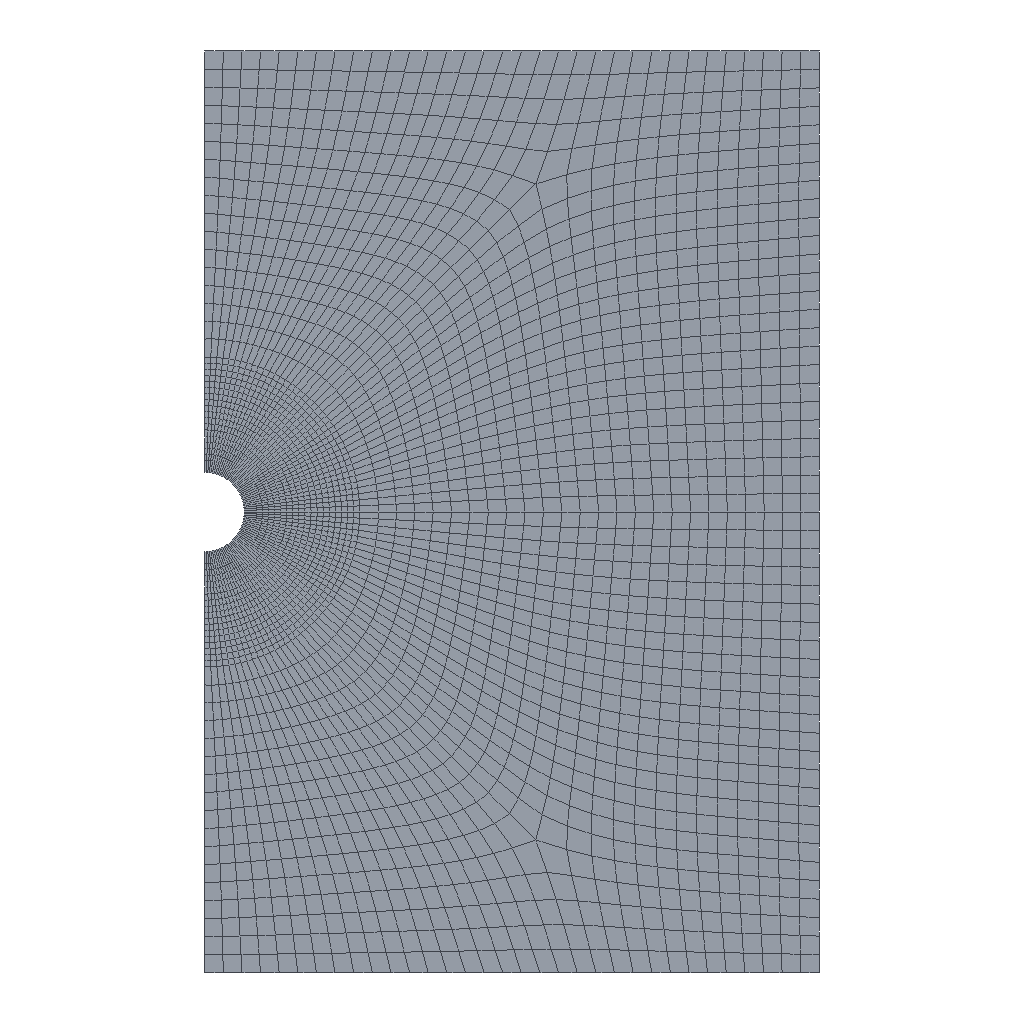Simulation study | abaqus
Set-up summary:
category,name,step,type,value,unit,region
solver,abaqus
solver,version,,,Abaqus/Standard 2020
units,not stated in the deck,,not stated
analysis,deck,,geostatic,geostatic
load_step,geo,geo,geostatic
load_step,Step-1,Step-1,soils
load_step,requested,,,2
mesh,nodes,,,3503
mesh,elements,,,3349
element_type,CPE4P,,plane,3330
element_type,COH2D4P,,cohesive,19
load,load commands in deck,,count,4
bc,support commands in deck,,count,4
material,COH,,in results
material,COH-0,,in results
material,ROCK,,in results
check,setup vs results,,match,"per instance, exact: element labels, types and connectivity; labels of the nodes the elements use; coordinates of those nodes at SINGLE_PRECISION in 1 of 1 instance(s)"
Abaqus input file, long lists of numbers shortened:
*Heading
** Job name: Job-2 Model name: Model-1-Copy-Copy
** Generated by: Abaqus/CAE 2020
*Preprint, echo=NO, model=NO, history=NO, contact=NO
**
** PARTS
**
*Part, name=work
*Node
      1,   25.206,           0.
      2,   6.441,           0.
** (3501 more lines like these left out)
*Element, type=CPE4P
  1,    1, 3466,  390,  125
  2, 3466, 3467,  391,  390
** (3328 more lines like these left out)
*Element, type=COH2D4P
3331,    1,   12, 3466,    1,    1, 3485
3332,   12,   13, 3467, 3466, 3485, 3486
** (17 more lines like these left out)
*Nset, nset=Set-111
    1,    2,    3,    4,    5,    6,   12,   13,   14,   15,   16,   17,   18,   19,   20,   21
   22,   23,   24,   25,   26,   27,   28,   29,   30,   31,   32,   33,   34,   35,   36,   37
** (101 more lines like these left out)
*Elset, elset=Set-111, generate
    1,  1520,     1
*Nset, nset=Set-120, generate
    1,  3484,     1
*Elset, elset=Set-120, generate
    1,  3330,     1
*Nset, nset=CohesiveSeam-2-TopNodes
    1, 3466, 3467, 3468, 3469, 3470, 3471, 3472, 3473, 3474, 3475, 3476, 3477, 3478, 3479, 3480
 3481, 3482, 3483, 3484
*Nset, nset=CohesiveSeam-2-BottomNodes
  1,  2, 12, 13, 14, 15, 16, 17, 18, 19, 20, 21, 22, 23, 24, 25
 26, 27, 28, 29
*Nset, nset=CohesiveSeam-2-MidNodes
    1, 3485, 3486, 3487, 3488, 3489, 3490, 3491, 3492, 3493, 3494, 3495, 3496, 3497, 3498, 3499
 3500, 3501, 3502, 3503
*Elset, elset=ele-3336-plug
 3336,
*Nset, nset=node-weiyi-0
   17, 3471, 3490
*Elset, elset=coh-shengyu
 3331, 3332, 3333, 3334, 3335, 3337, 3338, 3339, 3340, 3341, 3342, 3343, 3344, 3345, 3346, 3347
 3348, 3349
*Nset, nset=node-inject
 3503,
*Elset, elset=CohesiveSeam-2-Elements, generate
 3331,  3349,     1
*Elset, elset=Set-qilie
 3349,
*Elset, elset=Set-pore-pressure, generate
 775,  779,    1
*Elset, elset=pressure, generate
 10,  19,   1
*Nset, nset=Set-14
   12,   13,   14,   15,   16, 3466, 3467, 3468, 3469, 3470
*Nset, nset=Set-press
    2,   20,   21,   22,   23,   24,   25,   26,   27,   28,   29, 3474, 3475, 3476, 3477, 3478
 3479, 3480, 3481, 3482, 3483, 3484
*Elset, elset=__PickedSurf167_S3, internal, generate
 742,  760,    1
*Surface, type=ELEMENT, name=_PickedSurf167, internal
__PickedSurf167_S3, S3
*Elset, elset=__PickedSurf206_S3, internal, generate
 3331,  3349,     1
*Surface, type=ELEMENT, name=_PickedSurf206, internal
__PickedSurf206_S3, S3
*Elset, elset=_CohesiveSeam-2-TopSurf_S3, internal, generate
 3331,  3349,     1
*Surface, type=ELEMENT, name=CohesiveSeam-2-TopSurf
_CohesiveSeam-2-TopSurf_S3, S3
*Elset, elset=_CohesiveSeam-2-BottomSurf_S1, internal, generate
 3331,  3349,     1
*Surface, type=ELEMENT, name=CohesiveSeam-2-BottomSurf
_CohesiveSeam-2-BottomSurf_S1, S1
** Section: rock
*Solid Section, elset=Set-120, material=rock
,
** Section: coh
*Cohesive Section, elset=CohesiveSeam-2-Elements, material=coh, response=TRACTION SEPARATION, thickness=SPECIFIED
0.001,
*End Part
**
**
** ASSEMBLY
**
*Assembly, name=Assembly
**
*Instance, name=work-1, part=work
*Nset, nset=Set-14_PP_, internal
   12,   13,   14,   15,   16, 3466, 3467, 3468, 3469, 3470
*End Instance
**
*Nset, nset=Set-3, instance=work-1
   3,   4,   5,   6,  69,  70,  71,  72,  73,  74,  75,  76,  77,  78,  79,  80
  81,  82,  83,  84,  85,  86, 165, 166, 167, 168, 169, 170, 171, 172, 173, 174
** (1 more lines like these left out)
*Elset, elset=Set-3, instance=work-1
  742,  743,  744,  745,  746,  747,  748,  749,  750,  751,  752,  753,  754,  755,  756,  757
  758,  759,  760, 1502, 1503, 1504, 1505, 1506, 1507, 1508, 1509, 1510, 1511, 1512, 1513, 1514
** (1 more lines like these left out)
*Nset, nset=Set-4, instance=work-1
   7,   9, 222, 223, 224, 225, 226, 227, 228, 229, 230, 231, 232, 233, 234, 235
 236, 237, 238, 239, 240, 241, 242, 243, 244, 245
*Elset, elset=Set-4, instance=work-1
 1521, 1522, 1523, 1524, 1525, 1526, 1527, 1528, 1529, 1530, 1531, 1532, 1533, 1534, 1535, 1536
 1537, 1538, 1539, 1540, 2373, 2386, 2399, 2412, 2425
*Nset, nset=Set-5, instance=work-1
   8,   9, 286, 287, 288, 289, 290, 291, 292, 293, 294, 295, 296, 297, 298, 299
 300, 301, 302, 303, 304, 305, 306, 307, 308, 309, 310, 311, 312, 313, 314, 315
** (1 more lines like these left out)
*Elset, elset=Set-5, instance=work-1
 2265, 2270, 2275, 2280, 2285, 2290, 2295, 2300, 2305, 2310, 2315, 2320, 2325, 2330, 2335, 2340
 2345, 2350, 2355, 2360, 2361, 2362, 2363, 2364, 2365, 2366, 2367, 2368, 2369, 2370, 2371, 2372
** (1 more lines like these left out)
*Nset, nset=Set-12, instance=work-1
   7,   9, 222, 223, 224, 225, 226, 227, 228, 229, 230, 231, 232, 233, 234, 235
 236, 237, 238, 239, 240, 241, 242, 243, 244, 245
*Elset, elset=Set-12, instance=work-1
 1521, 1522, 1523, 1524, 1525, 1526, 1527, 1528, 1529, 1530, 1531, 1532, 1533, 1534, 1535, 1536
 1537, 1538, 1539, 1540, 2373, 2386, 2399, 2412, 2425
*Nset, nset=Set-13, instance=work-1
   8,   9, 286, 287, 288, 289, 290, 291, 292, 293, 294, 295, 296, 297, 298, 299
 300, 301, 302, 303, 304, 305, 306, 307, 308, 309, 310, 311, 312, 313, 314, 315
** (1 more lines like these left out)
*Elset, elset=Set-13, instance=work-1
 2265, 2270, 2275, 2280, 2285, 2290, 2295, 2300, 2305, 2310, 2315, 2320, 2325, 2330, 2335, 2340
 2345, 2350, 2355, 2360, 2361, 2362, 2363, 2364, 2365, 2366, 2367, 2368, 2369, 2370, 2371, 2372
** (1 more lines like these left out)
*Nset, nset=Set-14, instance=work-1
    1,    2,    3,    4,    5,    6,    7,    8,    9,   12,   13,   14,   15,   16,   17,   18
   19,   20,   21,   22,   23,   24,   25,   26,   27,   28,   29,   30,   31,   32,   33,   34
** (105 more lines like these left out)
*Elset, elset=Set-14, instance=work-1
    1,    2,    3,    4,    5,    6,    7,    8,    9,   10,   11,   12,   13,   14,   15,   16
   17,   18,   19,   20,   21,   22,   23,   24,   25,   26,   27,   28,   29,   30,   31,   32
** (97 more lines like these left out)
*Nset, nset=Set-15, instance=work-1
    1,    2,    3,    4,    5,    6,   12,   13,   14,   15,   16,   17,   18,   19,   20,   21
   22,   23,   24,   25,   26,   27,   28,   29,   30,   31,   32,   33,   34,   35,   36,   37
** (101 more lines like these left out)
*Elset, elset=Set-15, instance=work-1, generate
    1,  1520,     1
*Nset, nset=Set-16, instance=work-1
   3,   4,   5,   6,  69,  70,  71,  72,  73,  74,  75,  76,  77,  78,  79,  80
  81,  82,  83,  84,  85,  86, 165, 166, 167, 168, 169, 170, 171, 172, 173, 174
** (1 more lines like these left out)
*Elset, elset=Set-16, instance=work-1
  742,  743,  744,  745,  746,  747,  748,  749,  750,  751,  752,  753,  754,  755,  756,  757
  758,  759,  760, 1502, 1503, 1504, 1505, 1506, 1507, 1508, 1509, 1510, 1511, 1512, 1513, 1514
** (1 more lines like these left out)
*Nset, nset=Set-17, instance=work-1
    3,   30,   31,   32,   33,   34,   35,   36,   37,   38,   39,   40,   41,   42,   43,   44
   45,   46,   47,   48,   49,   50,   51,   52,   53,   54,   55,   56,   57,   58,   59,   60
** (1 more lines like these left out)
*Elset, elset=Set-17, instance=work-1, generate
  19,  760,   19
*Nset, nset=Set-18, instance=work-1
   3,   4,   5,   6,   8,  11,  69,  70,  71,  72,  73,  74,  75,  76,  77,  78
  79,  80,  81,  82,  83,  84,  85,  86, 165, 166, 167, 168, 169, 170, 171, 172
** (3 more lines like these left out)
*Elset, elset=Set-18, instance=work-1
  742,  743,  744,  745,  746,  747,  748,  749,  750,  751,  752,  753,  754,  755,  756,  757
  758,  759,  760, 1502, 1503, 1504, 1505, 1506, 1507, 1508, 1509, 1510, 1511, 1512, 1513, 1514
** (3 more lines like these left out)
*Nset, nset=Set-19, instance=work-1
   7,   9,  10, 222, 223, 224, 225, 226, 227, 228, 229, 230, 231, 232, 233, 234
 235, 236, 237, 238, 239, 240, 241, 242, 243, 244, 245, 318, 319, 320, 321, 322
** (2 more lines like these left out)
*Elset, elset=Set-19, instance=work-1
 1521, 1522, 1523, 1524, 1525, 1526, 1527, 1528, 1529, 1530, 1531, 1532, 1533, 1534, 1535, 1536
 1537, 1538, 1539, 1540, 2373, 2386, 2399, 2412, 2425, 2678, 2691, 2704, 2717, 2730, 2743, 2756
** (2 more lines like these left out)
*Nset, nset=Set-20, instance=work-1
   8,   9,  10,  11, 286, 287, 288, 289, 290, 291, 292, 293, 294, 295, 296, 297
 298, 299, 300, 301, 302, 303, 304, 305, 306, 307, 308, 309, 310, 311, 312, 313
** (3 more lines like these left out)
*Elset, elset=Set-20, instance=work-1
 2265, 2270, 2275, 2280, 2285, 2290, 2295, 2300, 2305, 2310, 2315, 2320, 2325, 2330, 2335, 2340
 2345, 2350, 2355, 2360, 2361, 2362, 2363, 2364, 2365, 2366, 2367, 2368, 2369, 2370, 2371, 2372
** (3 more lines like these left out)
*Nset, nset=Set-21, instance=work-1, generate
    1,  3484,     1
*Elset, elset=Set-21, instance=work-1, generate
    1,  3349,     1
*Nset, nset=Set-22, instance=work-1, generate
    1,  3484,     1
*Elset, elset=Set-22, instance=work-1, generate
    1,  3330,     1
*Elset, elset=_Surf-12_S2, internal, instance=work-1, generate
  19,  760,   19
*Surface, type=ELEMENT, name=Surf-12
_Surf-12_S2, S2
*Elset, elset=_Surf-14_S2, internal, instance=work-1, generate
  19,  760,   19
*Elset, elset=_Surf-14_S4, internal, instance=work-1, generate
  761,  1502,    19
*Surface, type=ELEMENT, name=Surf-14
_Surf-14_S2, S2
_Surf-14_S4, S4
*End Assembly
*Amplitude, name=Amp-1
             0.,              0.,             50.,              1.
**
** MATERIALS
**
*Material, name=coh
*Damage Initiation, criterion=MAXS
 1e+06,  5e+06,500000.
*Damage Evolution, type=DISPLACEMENT
 1e-09,
*Elastic, type=TRACTION
 1.5e+10, 1.5e+10, 1.5e+10
*Fluid Leakoff
 1e-14, 1e-14
*Gap Flow
 0.001,
*Material, name=coh-0
*Damage Initiation, criterion=MAXS
 1e+06, 5e+06, 5e+06
*Damage Evolution, type=DISPLACEMENT
 1e-09,
*Elastic, type=TRACTION
 1.5e+10, 1.5e+10, 1.5e+10
*Gap Flow
 1e-50,
*Material, name=rock
*Elastic
 1.5e+10, 0.25
*Permeability, specific=9800.
 1e-07, 0.2
**
** INTERACTION PROPERTIES
**
*Surface Interaction, name=IntProp-1
1.,
**
** BOUNDARY CONDITIONS
**
** Name: [REDACTED] : Displacement/rotation angle
*Boundary
Set-19, 1, 1
** Name: [REDACTED] : Symmetric / antisymmetric / fully fixed
*Boundary
Set-18, XSYMM
** Name: [REDACTED] : Displacement/rotation angle
*Boundary
Set-20, 2, 2
**
** PREDEFINED FIELDS
**
** Name: Predefined Field-1   Type: Void ratio
*Initial Conditions, TYPE=RATIO
Set-21, 0.2
** Name: Predefined Field-2   Type: Stress
*Initial Conditions, type=STRESS
Set-22, -1e+06, -1e+06, -1e+06, 0.,
** ----------------------------------------------------------------
*initial conditions,type=initial gap
work-1.Set-qilie
**
** STEP: geo
**
*Step, name=geo, nlgeom=NO, unsymm=YES
*Geostatic
**
** CONTROLS
**
*Controls, reset
*Controls, parameters=time incrementation
, , , , , , , 20, , ,
**
** OUTPUT REQUESTS
**
*Restart, write, frequency=0
**
** FIELD OUTPUT: F-Output-1
**
*Output, field
*Node Output
CF, PHILSM, POR, PSILSM, RF, U
*Element Output, directions=YES
E, FLUVR, FLVEL, LE, LOADSXFEM, MISES, PFOPENXFEM, S, SAT, SDEG, VOIDR,pfopen
*Contact Output
CSDMG, PFL, PFLA, PTL, PTLA
*Output, history, frequency=0
*End Step
** ----------------------------------------------------------------
**
** STEP: Step-1
**
*Step, name=Step-1, nlgeom=YES, inc=10000, unsymm=YES
*Soils, consolidation, end=PERIOD, utol=1e+25, creep=none
0.01, 50., 3e-06, 50.,
**
** BOUNDARY CONDITIONS
**
** Name: BC-5 Type: 孔隙压力
*Boundary, amplitude=Amp-1
work-1.Set-14_PP_, 8, 8, 100000.
**
** LOADS
**
** Name: Load-2   Type: Pressure
*Dsload, amplitude=Amp-1
Surf-14, P, 1000.
** Name: Load-3   Type: Concentrated pore fluid
*Cflow, amplitude=Amp-1
work-1.node-inject,  , -0.005
** Name: Load-4   Type: Concentrated force
*Cload, amplitude=Amp-1
work-1.Set-press, 2, -1000.
**
** CONTROLS
**
*Controls, reset
*Controls, parameters=time incrementation
, , , , , , , 20, , ,
**
** OUTPUT REQUESTS
**
*Restart, write, frequency=0
**
** FIELD OUTPUT: F-Output-1
**
*Output, field
*Node Output
CF, PHILSM, POR, PSILSM, RF, U
*Element Output, directions=YES
E, FLUVR, FLVEL, LE, MISES, S, SAT, SDEG, VOIDR,pfopen
*Contact Output
CSDMG, PFL, PFLA, PTL, PTLA
**
** HISTORY OUTPUT: H-Output-1
**
*Output, history
*Node Output, nset=work-1.node-inject
POR,
*End Step
Results summary:
result,step,,completed,increments=1 time=1.0/1.0
result,step,,completed,increments=34 time=50.0/50.0
result,analysis,,,"soils, consolidation"
result,last_loadstep,,,2
result,primary field,,,"U, POR"
result,reaction total,,FX,-12869.0,model units
result,reaction total,,FY,22000.0,model units
result,reaction total,,FZ,0.0,model units